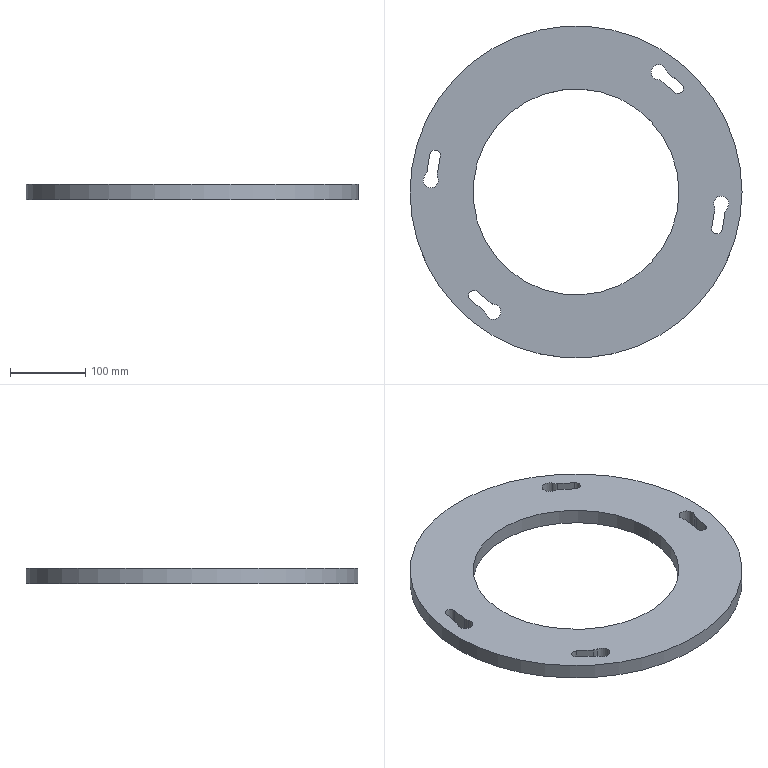NC program | NX | posted with a generic post | part box 440 x 440 x 20 mm
Lines 6893 to 7039 of 7039:
(ZLEVEL_PROFILE_COPY , TOOL : D10JING)
N13784 T09 M6
N13786 G54
N13788 G17 G0 G90 X-187.538 Y49.287 S5000 M3
N13790 G43 Z80. H9
N13792 Z-17.
N13794 G94 G1 Z-20. F1200.
N13796 X-188.102 Y49.753
N13798 G3 X-188.74 Y48.983 R1.
N13800 G1 X-192.456 Y27.011
N13802 G2 X-196.253 Y18.638 R18.
N13804 G3 X-187.68 Y17.188 R-5.
N13806 G2 X-188.512 Y26.344 R18.
N13808 G1 X-184.796 Y48.316
N13810 G3 X-186.434 Y50.621 R2.
N13812 X-188.74 Y48.983 R2.
N13814 X-188.391 Y48.046 R1.
N13816 G1 X-187.946 Y47.678
N13818 Z-17.
N13820 G0 Z80.
N13822 X-136.453 Y-137.77
N13824 Z-17.
N13826 G1 Z-20.
N13828 X-137.139 Y-138.025
N13830 G3 X-136.79 Y-138.962 R1.
N13832 G1 X-119.62 Y-153.167
N13834 G2 X-114.268 Y-160.642 R18.
N13836 G3 X-108.725 Y-153.941 R-5.
N13838 G2 X-117.07 Y-150.085 R18.
N13840 G1 X-134.241 Y-135.88
N13842 G3 X-137.057 Y-136.146 R2.
N13844 X-136.79 Y-138.962 R2.
N13846 X-135.804 Y-139.129 R1.
N13848 G1 X-135.263 Y-138.928
N13850 Z-17.
N13852 G0 Z80.
N13854 X187.538 Y-49.287
N13856 Z-17.
N13858 G1 Z-20.
N13860 X188.102 Y-49.753
N13862 G3 X188.74 Y-48.983 R1.
N13864 G1 X192.456 Y-27.011
N13866 G2 X196.253 Y-18.638 R18.
N13868 G3 X187.68 Y-17.188 R-5.
N13870 G2 X188.512 Y-26.344 R18.
N13872 G1 X184.796 Y-48.316
N13874 G3 X186.434 Y-50.621 R2.
N13876 X188.74 Y-48.983 R2.
N13878 X188.391 Y-48.046 R1.
N13880 G1 X187.946 Y-47.678
N13882 Z-17.
N13884 G0 Z80.
N13886 X136.453 Y137.77
N13888 Z-17.
N13890 G1 Z-20.
N13892 X137.139 Y138.025
N13894 G3 X136.79 Y138.962 R1.
N13896 G1 X119.62 Y153.167
N13898 G2 X114.268 Y160.642 R18.
N13900 G3 X108.725 Y153.941 R-5.
N13902 G2 X117.07 Y150.085 R18.
N13904 G1 X134.241 Y135.88
N13906 G3 X137.057 Y136.146 R2.
N13908 X136.79 Y138.962 R2.
N13910 X135.804 Y139.129 R1.
N13912 G1 X135.263 Y138.928
N13914 Z-17.
N13916 G0 Z80.
N13918 M5
(ZLEVEL_PROFILE_COPY_COPY , TOOL : D6A45)
N13920 T07 M6
N13922 G54
N13924 G17 G0 G90 X130.844 Y147.623 S7500 M3
N13926 G43 Z80. H7
N13928 Z2.
N13930 G94 G1 Z-1. F1200.
N13932 X131.017 Y148.648
N13934 G3 X130.808 Y149.21 R0.6
N13936 G1 X122.223 Y156.312
N13938 G2 X118.084 Y162.092 R13.917
N13940 G3 X108.015 Y149.921 R-9.083
N13942 G2 X114.468 Y146.939 R13.917
N13944 G1 X131.638 Y132.734
N13946 G3 X140.202 Y133.544 R6.083
N13948 X139.393 Y142.108 R6.083
N13950 G1 X130.808 Y149.21
N13952 G3 X130.216 Y149.31 R0.6
N13954 G1 X129.242 Y148.948
N13956 Z2.
N13958 G0 Z80.
N13960 X-130.844 Y-147.623
N13962 Z2.
N13964 G1 Z-1.
N13966 X-131.017 Y-148.648
N13968 G3 X-130.808 Y-149.21 R0.6
N13970 G1 X-122.223 Y-156.312
N13972 G2 X-118.084 Y-162.092 R13.917
N13974 G3 X-108.015 Y-149.921 R-9.083
N13976 G2 X-114.468 Y-146.939 R13.917
N13978 G1 X-131.638 Y-132.734
N13980 G3 X-140.202 Y-133.544 R6.083
N13982 X-139.393 Y-142.108 R6.083
N13984 G1 X-130.808 Y-149.21
N13986 G3 X-130.216 Y-149.31 R0.6
N13988 G1 X-129.242 Y-148.948
N13990 Z2.
N13992 G0 Z80.
N13994 X193.267 Y-39.502
N13996 Z2.
N13998 G1 Z-1.
N14000 X194.241 Y-39.14
N14002 G3 X194.624 Y-38.678 R0.6
N14004 G1 X196.482 Y-27.692
N14006 G2 X199.418 Y-21.218 R13.917
N14008 G3 X183.843 Y-18.584 R-9.083
N14010 G2 X184.487 Y-25.663 R13.917
N14012 G1 X180.77 Y-47.635
N14014 G3 X185.753 Y-54.647 R6.083
N14016 X192.766 Y-49.664 R6.083
N14018 G1 X194.624 Y-38.678
N14020 G3 X194.415 Y-38.115 R0.6
N14022 G1 X193.614 Y-37.453
N14024 Z2.
N14026 G0 Z80.
N14028 X-193.267 Y39.502
N14030 Z2.
N14032 G1 Z-1.
N14034 X-194.241 Y39.14
N14036 G3 X-194.624 Y38.678 R0.6
N14038 G1 X-196.482 Y27.692
N14040 G2 X-199.418 Y21.218 R13.917
N14042 G3 X-183.843 Y18.584 R-9.083
N14044 G2 X-184.487 Y25.663 R13.917
N14046 G1 X-180.77 Y47.635
N14048 G3 X-185.753 Y54.647 R6.083
N14050 X-192.766 Y49.664 R6.083
N14052 G1 X-194.624 Y38.678
N14054 G3 X-194.415 Y38.115 R0.6
N14056 G1 X-193.614 Y37.453
N14058 Z2.
N14060 G0 Z80.
N14062 M5
N14064 M2